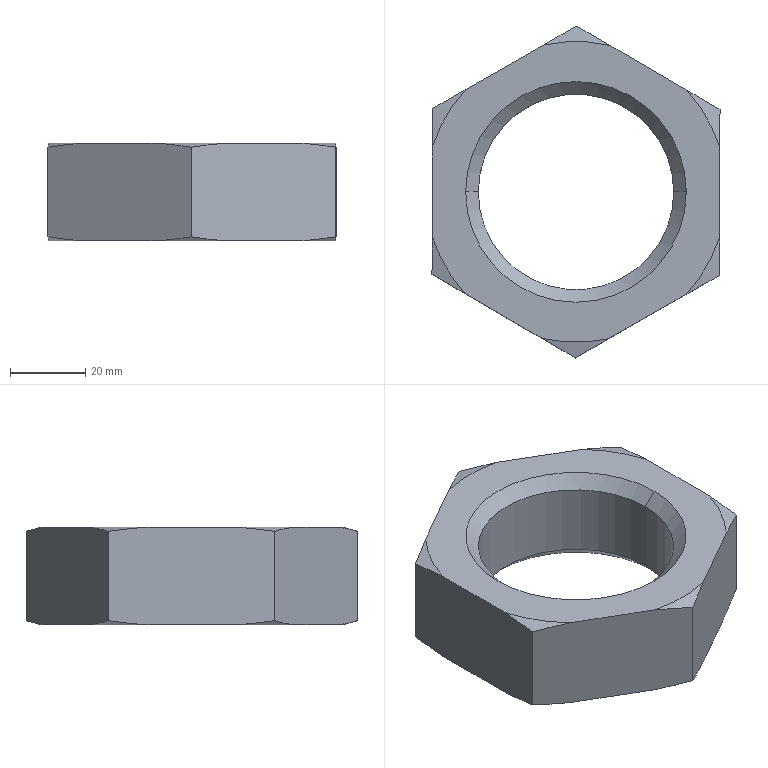Part | SolidWorks | features Cut 2, Chamfer 1, Extrusion 1 | 1 solid | 26 faces | box 76.6 x 88.249 x 26 mm | volume 74263 mm3 | cone 16 | plane 8 | cylinder 2 | commonest cylinder face diameters 52 x2
STEP:
#1=CARTESIAN_POINT('',(-26.,0.,22.662));
#2=VERTEX_POINT('',#1);
#3=CARTESIAN_POINT('',(26.,0.,22.662));
#4=VERTEX_POINT('',#3);
#5=CARTESIAN_POINT('',(0.,0.,22.662));
#6=DIRECTION('',(0.,0.,1.));
#7=DIRECTION('',(-1.,0.,0.));
#8=AXIS2_PLACEMENT_3D('',#5,#6,#7);
#9=CIRCLE('',#8,26.);
#10=EDGE_CURVE('',#2,#4,#9,.T.);
#11=ORIENTED_EDGE('',*,*,#10,.F.);
#12=CARTESIAN_POINT('',(-29.338,0.,26.));
#13=VERTEX_POINT('',#12);
#14=CARTESIAN_POINT('',(-26.,0.,22.662));
#15=DIRECTION('',(-0.7071,0.,0.7071));
#16=VECTOR('',#15,1000.);
#17=LINE('',#14,#16);
#18=EDGE_CURVE('',#2,#13,#17,.T.);
#19=ORIENTED_EDGE('',*,*,#18,.T.);
#20=CARTESIAN_POINT('',(29.338,0.,26.));
#21=VERTEX_POINT('',#20);
#22=CARTESIAN_POINT('',(0.,0.,26.));
#23=DIRECTION('',(0.,0.,-1.));
#24=DIRECTION('',(-1.,0.,0.));
#25=AXIS2_PLACEMENT_3D('',#22,#23,#24);
#26=CIRCLE('',#25,29.338);
#27=EDGE_CURVE('',#21,#13,#26,.T.);
#28=ORIENTED_EDGE('',*,*,#27,.F.);
#29=CARTESIAN_POINT('',(26.,0.,22.662));
#30=DIRECTION('',(0.7071,0.,0.7071));
#31=VECTOR('',#30,1000.);
#32=LINE('',#29,#31);
#33=EDGE_CURVE('',#4,#21,#32,.T.);
#34=ORIENTED_EDGE('',*,*,#33,.F.);
#35=EDGE_LOOP('',(#11,#19,#28,#34));
#36=FACE_OUTER_BOUND('',#35,.T.);
#37=CARTESIAN_POINT('',(0.,0.,22.662));
#38=DIRECTION('',(0.,0.,1.));
#39=DIRECTION('',(1.,0.,0.));
#40=AXIS2_PLACEMENT_3D('',#37,#38,#39);
#41=CONICAL_SURFACE('',#40,26.,0.7854);
#42=ADVANCED_FACE('',(#36),#41,.F.);
#43=CARTESIAN_POINT('',(26.,0.,3.338));
#44=VERTEX_POINT('',#43);
#45=CARTESIAN_POINT('',(-26.,0.,3.338));
#46=VERTEX_POINT('',#45);
#47=CARTESIAN_POINT('',(0.,0.,3.338));
#48=DIRECTION('',(0.,0.,-1.));
#49=DIRECTION('',(-1.,0.,0.));
#50=AXIS2_PLACEMENT_3D('',#47,#48,#49);
#51=CIRCLE('',#50,26.);
#52=EDGE_CURVE('',#44,#46,#51,.T.);
#53=ORIENTED_EDGE('',*,*,#52,.F.);
#54=CARTESIAN_POINT('',(29.338,0.,0.));
#55=VERTEX_POINT('',#54);
#56=CARTESIAN_POINT('',(29.338,0.,0.));
#57=DIRECTION('',(0.7071,0.,-0.7071));
#58=VECTOR('',#57,1000.);
#59=LINE('',#56,#58);
#60=EDGE_CURVE('',#44,#55,#59,.T.);
#61=ORIENTED_EDGE('',*,*,#60,.T.);
#62=CARTESIAN_POINT('',(-29.338,0.,0.));
#63=VERTEX_POINT('',#62);
#64=CARTESIAN_POINT('',(0.,0.,0.));
#65=DIRECTION('',(0.,0.,1.));
#66=DIRECTION('',(-1.,0.,0.));
#67=AXIS2_PLACEMENT_3D('',#64,#65,#66);
#68=CIRCLE('',#67,29.338);
#69=EDGE_CURVE('',#63,#55,#68,.T.);
#70=ORIENTED_EDGE('',*,*,#69,.F.);
#71=CARTESIAN_POINT('',(-29.338,0.,0.));
#72=DIRECTION('',(-0.7071,0.,-0.7071));
#73=VECTOR('',#72,1000.);
#74=LINE('',#71,#73);
#75=EDGE_CURVE('',#46,#63,#74,.T.);
#76=ORIENTED_EDGE('',*,*,#75,.F.);
#77=EDGE_LOOP('',(#53,#61,#70,#76));
#78=FACE_OUTER_BOUND('',#77,.T.);
#79=CARTESIAN_POINT('',(0.,0.,0.));
#80=DIRECTION('',(0.,0.,-1.));
#81=DIRECTION('',(-1.,0.,0.));
#82=AXIS2_PLACEMENT_3D('',#79,#80,#81);
#83=CONICAL_SURFACE('',#82,29.338,0.7854);
#84=ADVANCED_FACE('',(#78),#83,.F.);
#85=ORIENTED_EDGE('',*,*,#10,.T.);
#86=CARTESIAN_POINT('',(26.,0.,26.));
#87=DIRECTION('',(0.,0.,-1.));
#88=VECTOR('',#87,1000.);
#89=LINE('',#86,#88);
#90=EDGE_CURVE('',#4,#44,#89,.T.);
#91=ORIENTED_EDGE('',*,*,#90,.T.);
#92=ORIENTED_EDGE('',*,*,#52,.T.);
#93=CARTESIAN_POINT('',(-26.,0.,26.));
#94=DIRECTION('',(0.,0.,-1.));
#95=VECTOR('',#94,1000.);
#96=LINE('',#93,#95);
#97=EDGE_CURVE('',#2,#46,#96,.T.);
#98=ORIENTED_EDGE('',*,*,#97,.F.);
#99=EDGE_LOOP('',(#85,#91,#92,#98));
#100=FACE_OUTER_BOUND('',#99,.T.);
#101=CARTESIAN_POINT('',(0.,0.,26.));
#102=DIRECTION('',(0.,0.,-1.));
#103=DIRECTION('',(-1.,0.,0.));
#104=AXIS2_PLACEMENT_3D('',#101,#102,#103);
#105=CYLINDRICAL_SURFACE('',#104,26.);
#106=ADVANCED_FACE('',(#100),#105,.F.);
#107=CARTESIAN_POINT('',(38.3,21.912,24.895));
#108=VERTEX_POINT('',#107);
#109=CARTESIAN_POINT('',(29.451,27.068,26.));
#110=VERTEX_POINT('',#109);
#111=CARTESIAN_POINT('',(38.3,21.912,24.895));
#112=CARTESIAN_POINT('',(35.358,23.626,25.351));
#113=CARTESIAN_POINT('',(32.41,25.344,25.729));
#114=CARTESIAN_POINT('',(29.451,27.068,26.));
#115=B_SPLINE_CURVE_WITH_KNOTS('',3,(#111,#112,#113,#114),.UNSPECIFIED.,.F.,.F.,(4,4),(0.03608,0.04638),.UNSPECIFIED.);
#116=EDGE_CURVE('',#108,#110,#115,.T.);
#117=ORIENTED_EDGE('',*,*,#116,.F.);
#118=CARTESIAN_POINT('',(38.3,21.912,1.105));
#119=VERTEX_POINT('',#118);
#120=CARTESIAN_POINT('',(38.3,21.912,26.));
#121=DIRECTION('',(0.,0.,-1.));
#122=VECTOR('',#121,1000.);
#123=LINE('',#120,#122);
#124=EDGE_CURVE('',#108,#119,#123,.T.);
#125=ORIENTED_EDGE('',*,*,#124,.T.);
#126=CARTESIAN_POINT('',(29.451,27.068,0.));
#127=VERTEX_POINT('',#126);
#128=CARTESIAN_POINT('',(29.451,27.068,0.));
#129=CARTESIAN_POINT('',(30.931,26.205,0.1356));
#130=CARTESIAN_POINT('',(32.411,25.343,0.2982));
#131=CARTESIAN_POINT('',(35.36,23.625,0.6692));
#132=CARTESIAN_POINT('',(36.831,22.768,0.8776));
#133=CARTESIAN_POINT('',(38.3,21.912,1.105));
#134=B_SPLINE_CURVE_WITH_KNOTS('',3,(#128,#129,#130,#131,#132,#133),.UNSPECIFIED.,.F.,.F.,(4,2,4),(0.06989,0.07495,0.08001),.UNSPECIFIED.);
#135=EDGE_CURVE('',#127,#119,#134,.T.);
#136=ORIENTED_EDGE('',*,*,#135,.F.);
#137=CARTESIAN_POINT('',(9.023,38.969,0.));
#138=VERTEX_POINT('',#137);
#139=CARTESIAN_POINT('',(38.3,21.912,0.));
#140=DIRECTION('',(-0.8641,0.5034,0.));
#141=VECTOR('',#140,1000.);
#142=LINE('',#139,#141);
#143=EDGE_CURVE('',#127,#138,#142,.T.);
#144=ORIENTED_EDGE('',*,*,#143,.T.);
#145=CARTESIAN_POINT('',(0.1736,44.125,1.105));
#146=VERTEX_POINT('',#145);
#147=CARTESIAN_POINT('',(0.1736,44.125,1.105));
#148=CARTESIAN_POINT('',(3.115,42.411,0.6492));
#149=CARTESIAN_POINT('',(6.064,40.693,0.2712));
#150=CARTESIAN_POINT('',(9.023,38.969,0.));
#151=B_SPLINE_CURVE_WITH_KNOTS('',3,(#147,#148,#149,#150),.UNSPECIFIED.,.F.,.F.,(4,4),(0.03608,0.04638),.UNSPECIFIED.);
#152=EDGE_CURVE('',#146,#138,#151,.T.);
#153=ORIENTED_EDGE('',*,*,#152,.F.);
#154=CARTESIAN_POINT('',(0.1736,44.125,24.895));
#155=VERTEX_POINT('',#154);
#156=CARTESIAN_POINT('',(0.1736,44.125,26.));
#157=DIRECTION('',(0.,0.,-1.));
#158=VECTOR('',#157,1000.);
#159=LINE('',#156,#158);
#160=EDGE_CURVE('',#155,#146,#159,.T.);
#161=ORIENTED_EDGE('',*,*,#160,.F.);
#162=CARTESIAN_POINT('',(9.023,38.969,26.));
#163=VERTEX_POINT('',#162);
#164=CARTESIAN_POINT('',(9.023,38.969,26.));
#165=CARTESIAN_POINT('',(7.543,39.831,25.864));
#166=CARTESIAN_POINT('',(6.063,40.693,25.702));
#167=CARTESIAN_POINT('',(3.113,42.412,25.331));
#168=CARTESIAN_POINT('',(1.642,43.269,25.122));
#169=CARTESIAN_POINT('',(0.1736,44.125,24.895));
#170=B_SPLINE_CURVE_WITH_KNOTS('',3,(#164,#165,#166,#167,#168,#169),.UNSPECIFIED.,.F.,.F.,(4,2,4),(0.06989,0.07495,0.08001),.UNSPECIFIED.);
#171=EDGE_CURVE('',#163,#155,#170,.T.);
#172=ORIENTED_EDGE('',*,*,#171,.F.);
#173=CARTESIAN_POINT('',(38.3,21.912,26.));
#174=DIRECTION('',(-0.8641,0.5034,0.));
#175=VECTOR('',#174,1000.);
#176=LINE('',#173,#175);
#177=EDGE_CURVE('',#110,#163,#176,.T.);
#178=ORIENTED_EDGE('',*,*,#177,.F.);
#179=EDGE_LOOP('',(#117,#125,#136,#144,#153,#161,#172,#178));
#180=FACE_OUTER_BOUND('',#179,.T.);
#181=CARTESIAN_POINT('',(38.3,21.912,26.));
#182=DIRECTION('',(-0.5034,-0.8641,0.));
#183=DIRECTION('',(0.8641,-0.5034,0.));
#184=AXIS2_PLACEMENT_3D('',#181,#182,#183);
#185=PLANE('',#184);
#186=ADVANCED_FACE('',(#180),#185,.F.);
#187=CARTESIAN_POINT('',(-8.716,39.039,26.));
#188=VERTEX_POINT('',#187);
#189=CARTESIAN_POINT('',(0.1736,44.125,24.895));
#190=CARTESIAN_POINT('',(-2.781,42.434,25.351));
#191=CARTESIAN_POINT('',(-5.743,40.739,25.729));
#192=CARTESIAN_POINT('',(-8.716,39.039,26.));
#193=B_SPLINE_CURVE_WITH_KNOTS('',3,(#189,#190,#191,#192),.UNSPECIFIED.,.F.,.F.,(4,4),(0.03592,0.04622),.UNSPECIFIED.);
#194=EDGE_CURVE('',#155,#188,#193,.T.);
#195=ORIENTED_EDGE('',*,*,#194,.F.);
#196=ORIENTED_EDGE('',*,*,#160,.T.);
#197=CARTESIAN_POINT('',(-8.716,39.039,0.));
#198=VERTEX_POINT('',#197);
#199=CARTESIAN_POINT('',(-8.716,39.039,0.));
#200=CARTESIAN_POINT('',(-7.229,39.889,0.1356));
#201=CARTESIAN_POINT('',(-5.743,40.74,0.2982));
#202=CARTESIAN_POINT('',(-2.78,42.435,0.6692));
#203=CARTESIAN_POINT('',(-1.302,43.281,0.8776));
#204=CARTESIAN_POINT('',(0.1736,44.125,1.105));
#205=B_SPLINE_CURVE_WITH_KNOTS('',3,(#199,#200,#201,#202,#203,#204),.UNSPECIFIED.,.F.,.F.,(4,2,4),(0.06972,0.07478,0.07985),.UNSPECIFIED.);
#206=EDGE_CURVE('',#198,#146,#205,.T.);
#207=ORIENTED_EDGE('',*,*,#206,.F.);
#208=CARTESIAN_POINT('',(-29.237,27.298,0.));
#209=VERTEX_POINT('',#208);
#210=CARTESIAN_POINT('',(0.1736,44.125,0.));
#211=DIRECTION('',(-0.868,-0.4966,0.));
#212=VECTOR('',#211,1000.);
#213=LINE('',#210,#212);
#214=EDGE_CURVE('',#198,#209,#213,.T.);
#215=ORIENTED_EDGE('',*,*,#214,.T.);
#216=CARTESIAN_POINT('',(-38.126,22.213,1.105));
#217=VERTEX_POINT('',#216);
#218=CARTESIAN_POINT('',(-38.126,22.213,1.105));
#219=CARTESIAN_POINT('',(-35.171,23.903,0.6492));
#220=CARTESIAN_POINT('',(-32.209,25.598,0.2712));
#221=CARTESIAN_POINT('',(-29.237,27.298,0.));
#222=B_SPLINE_CURVE_WITH_KNOTS('',3,(#218,#219,#220,#221),.UNSPECIFIED.,.F.,.F.,(4,4),(0.03592,0.04622),.UNSPECIFIED.);
#223=EDGE_CURVE('',#217,#209,#222,.T.);
#224=ORIENTED_EDGE('',*,*,#223,.F.);
#225=CARTESIAN_POINT('',(-38.126,22.213,24.895));
#226=VERTEX_POINT('',#225);
#227=CARTESIAN_POINT('',(-38.126,22.213,26.));
#228=DIRECTION('',(0.,0.,-1.));
#229=VECTOR('',#228,1000.);
#230=LINE('',#227,#229);
#231=EDGE_CURVE('',#226,#217,#230,.T.);
#232=ORIENTED_EDGE('',*,*,#231,.F.);
#233=CARTESIAN_POINT('',(-29.237,27.298,26.));
#234=VERTEX_POINT('',#233);
#235=CARTESIAN_POINT('',(-29.237,27.298,26.));
#236=CARTESIAN_POINT('',(-30.723,26.448,25.864));
#237=CARTESIAN_POINT('',(-32.21,25.597,25.702));
#238=CARTESIAN_POINT('',(-35.173,23.902,25.331));
#239=CARTESIAN_POINT('',(-36.651,23.057,25.122));
#240=CARTESIAN_POINT('',(-38.126,22.213,24.895));
#241=B_SPLINE_CURVE_WITH_KNOTS('',3,(#235,#236,#237,#238,#239,#240),.UNSPECIFIED.,.F.,.F.,(4,2,4),(0.06972,0.07478,0.07985),.UNSPECIFIED.);
#242=EDGE_CURVE('',#234,#226,#241,.T.);
#243=ORIENTED_EDGE('',*,*,#242,.F.);
#244=CARTESIAN_POINT('',(0.1736,44.125,26.));
#245=DIRECTION('',(-0.868,-0.4966,0.));
#246=VECTOR('',#245,1000.);
#247=LINE('',#244,#246);
#248=EDGE_CURVE('',#188,#234,#247,.T.);
#249=ORIENTED_EDGE('',*,*,#248,.F.);
#250=EDGE_LOOP('',(#195,#196,#207,#215,#224,#232,#243,#249));
#251=FACE_OUTER_BOUND('',#250,.T.);
#252=CARTESIAN_POINT('',(0.1736,44.125,26.));
#253=DIRECTION('',(0.4966,-0.868,0.));
#254=DIRECTION('',(0.868,0.4966,0.));
#255=AXIS2_PLACEMENT_3D('',#252,#253,#254);
#256=PLANE('',#255);
#257=ADVANCED_FACE('',(#251),#256,.F.);
#258=CARTESIAN_POINT('',(-38.167,11.971,26.));
#259=VERTEX_POINT('',#258);
#260=CARTESIAN_POINT('',(-38.126,22.213,24.895));
#261=CARTESIAN_POINT('',(-38.14,18.808,25.351));
#262=CARTESIAN_POINT('',(-38.153,15.395,25.729));
#263=CARTESIAN_POINT('',(-38.167,11.971,26.));
#264=B_SPLINE_CURVE_WITH_KNOTS('',3,(#260,#261,#262,#263),.UNSPECIFIED.,.F.,.F.,(4,4),(0.03114,0.04144),.UNSPECIFIED.);
#265=EDGE_CURVE('',#226,#259,#264,.T.);
#266=ORIENTED_EDGE('',*,*,#265,.F.);
#267=ORIENTED_EDGE('',*,*,#231,.T.);
#268=CARTESIAN_POINT('',(-38.167,11.971,0.));
#269=VERTEX_POINT('',#268);
#270=CARTESIAN_POINT('',(-38.167,11.971,0.));
#271=CARTESIAN_POINT('',(-38.16,13.682,0.1355));
#272=CARTESIAN_POINT('',(-38.153,15.395,0.2981));
#273=CARTESIAN_POINT('',(-38.14,18.809,0.6691));
#274=CARTESIAN_POINT('',(-38.133,20.513,0.8775));
#275=CARTESIAN_POINT('',(-38.126,22.213,1.105));
#276=B_SPLINE_CURVE_WITH_KNOTS('',3,(#270,#271,#272,#273,#274,#275),.UNSPECIFIED.,.F.,.F.,(4,2,4),(0.06496,0.07003,0.0751),.UNSPECIFIED.);
#277=EDGE_CURVE('',#269,#217,#276,.T.);
#278=ORIENTED_EDGE('',*,*,#277,.F.);
#279=CARTESIAN_POINT('',(-38.26,-11.671,0.));
#280=VERTEX_POINT('',#279);
#281=CARTESIAN_POINT('',(-38.126,22.213,0.));
#282=DIRECTION('',(-0.003934,-1.,0.));
#283=VECTOR('',#282,1000.);
#284=LINE('',#281,#283);
#285=EDGE_CURVE('',#269,#280,#284,.T.);
#286=ORIENTED_EDGE('',*,*,#285,.T.);
#287=CARTESIAN_POINT('',(-38.3,-21.912,1.105));
#288=VERTEX_POINT('',#287);
#289=CARTESIAN_POINT('',(-38.3,-21.912,1.105));
#290=CARTESIAN_POINT('',(-38.286,-18.507,0.6491));
#291=CARTESIAN_POINT('',(-38.273,-15.094,0.2711));
#292=CARTESIAN_POINT('',(-38.26,-11.671,0.));
#293=B_SPLINE_CURVE_WITH_KNOTS('',3,(#289,#290,#291,#292),.UNSPECIFIED.,.F.,.F.,(4,4),(0.03114,0.04144),.UNSPECIFIED.);
#294=EDGE_CURVE('',#288,#280,#293,.T.);
#295=ORIENTED_EDGE('',*,*,#294,.F.);
#296=CARTESIAN_POINT('',(-38.3,-21.912,24.895));
#297=VERTEX_POINT('',#296);
#298=CARTESIAN_POINT('',(-38.3,-21.912,26.));
#299=DIRECTION('',(0.,0.,-1.));
#300=VECTOR('',#299,1000.);
#301=LINE('',#298,#300);
#302=EDGE_CURVE('',#297,#288,#301,.T.);
#303=ORIENTED_EDGE('',*,*,#302,.F.);
#304=CARTESIAN_POINT('',(-38.26,-11.671,26.));
#305=VERTEX_POINT('',#304);
#306=CARTESIAN_POINT('',(-38.26,-11.671,26.));
#307=CARTESIAN_POINT('',(-38.266,-13.381,25.865));
#308=CARTESIAN_POINT('',(-38.273,-15.095,25.702));
#309=CARTESIAN_POINT('',(-38.286,-18.509,25.331));
#310=CARTESIAN_POINT('',(-38.293,-20.212,25.122));
#311=CARTESIAN_POINT('',(-38.3,-21.912,24.895));
#312=B_SPLINE_CURVE_WITH_KNOTS('',3,(#306,#307,#308,#309,#310,#311),.UNSPECIFIED.,.F.,.F.,(4,2,4),(0.06496,0.07003,0.0751),.UNSPECIFIED.);
#313=EDGE_CURVE('',#305,#297,#312,.T.);
#314=ORIENTED_EDGE('',*,*,#313,.F.);
#315=CARTESIAN_POINT('',(-38.126,22.213,26.));
#316=DIRECTION('',(-0.003934,-1.,0.));
#317=VECTOR('',#316,1000.);
#318=LINE('',#315,#317);
#319=EDGE_CURVE('',#259,#305,#318,.T.);
#320=ORIENTED_EDGE('',*,*,#319,.F.);
#321=EDGE_LOOP('',(#266,#267,#278,#286,#295,#303,#314,#320));
#322=FACE_OUTER_BOUND('',#321,.T.);
#323=CARTESIAN_POINT('',(-38.126,22.213,26.));
#324=DIRECTION('',(1.,-0.003934,0.));
#325=DIRECTION('',(0.003934,1.,0.));
#326=AXIS2_PLACEMENT_3D('',#323,#324,#325);
#327=PLANE('',#326);
#328=ADVANCED_FACE('',(#322),#327,.F.);
#329=CARTESIAN_POINT('',(-29.451,-27.068,26.));
#330=VERTEX_POINT('',#329);
#331=CARTESIAN_POINT('',(-38.3,-21.912,24.895));
#332=CARTESIAN_POINT('',(-35.358,-23.626,25.351));
#333=CARTESIAN_POINT('',(-32.41,-25.344,25.729));
#334=CARTESIAN_POINT('',(-29.451,-27.068,26.));
#335=B_SPLINE_CURVE_WITH_KNOTS('',3,(#331,#332,#333,#334),.UNSPECIFIED.,.F.,.F.,(4,4),(0.03608,0.04638),.UNSPECIFIED.);
#336=EDGE_CURVE('',#297,#330,#335,.T.);
#337=ORIENTED_EDGE('',*,*,#336,.F.);
#338=ORIENTED_EDGE('',*,*,#302,.T.);
#339=CARTESIAN_POINT('',(-29.451,-27.068,0.));
#340=VERTEX_POINT('',#339);
#341=CARTESIAN_POINT('',(-29.451,-27.068,0.));
#342=CARTESIAN_POINT('',(-30.931,-26.205,0.1356));
#343=CARTESIAN_POINT('',(-32.411,-25.343,0.2982));
#344=CARTESIAN_POINT('',(-35.36,-23.625,0.6692));
#345=CARTESIAN_POINT('',(-36.831,-22.768,0.8776));
#346=CARTESIAN_POINT('',(-38.3,-21.912,1.105));
#347=B_SPLINE_CURVE_WITH_KNOTS('',3,(#341,#342,#343,#344,#345,#346),.UNSPECIFIED.,.F.,.F.,(4,2,4),(0.06989,0.07495,0.08001),.UNSPECIFIED.);
#348=EDGE_CURVE('',#340,#288,#347,.T.);
#349=ORIENTED_EDGE('',*,*,#348,.F.);
#350=CARTESIAN_POINT('',(-9.023,-38.969,0.));
#351=VERTEX_POINT('',#350);
#352=CARTESIAN_POINT('',(-38.3,-21.912,0.));
#353=DIRECTION('',(0.8641,-0.5034,0.));
#354=VECTOR('',#353,1000.);
#355=LINE('',#352,#354);
#356=EDGE_CURVE('',#340,#351,#355,.T.);
#357=ORIENTED_EDGE('',*,*,#356,.T.);
#358=CARTESIAN_POINT('',(-0.1736,-44.125,1.105));
#359=VERTEX_POINT('',#358);
#360=CARTESIAN_POINT('',(-0.1736,-44.125,1.105));
#361=CARTESIAN_POINT('',(-3.115,-42.411,0.6492));
#362=CARTESIAN_POINT('',(-6.064,-40.693,0.2712));
#363=CARTESIAN_POINT('',(-9.023,-38.969,0.));
#364=B_SPLINE_CURVE_WITH_KNOTS('',3,(#360,#361,#362,#363),.UNSPECIFIED.,.F.,.F.,(4,4),(0.03608,0.04638),.UNSPECIFIED.);
#365=EDGE_CURVE('',#359,#351,#364,.T.);
#366=ORIENTED_EDGE('',*,*,#365,.F.);
#367=CARTESIAN_POINT('',(-0.1736,-44.125,24.895));
#368=VERTEX_POINT('',#367);
#369=CARTESIAN_POINT('',(-0.1736,-44.125,26.));
#370=DIRECTION('',(0.,0.,-1.));
#371=VECTOR('',#370,1000.);
#372=LINE('',#369,#371);
#373=EDGE_CURVE('',#368,#359,#372,.T.);
#374=ORIENTED_EDGE('',*,*,#373,.F.);
#375=CARTESIAN_POINT('',(-9.023,-38.969,26.));
#376=VERTEX_POINT('',#375);
#377=CARTESIAN_POINT('',(-9.023,-38.969,26.));
#378=CARTESIAN_POINT('',(-7.543,-39.831,25.864));
#379=CARTESIAN_POINT('',(-6.063,-40.693,25.702));
#380=CARTESIAN_POINT('',(-3.113,-42.412,25.331));
#381=CARTESIAN_POINT('',(-1.642,-43.269,25.122));
#382=CARTESIAN_POINT('',(-0.1736,-44.125,24.895));
#383=B_SPLINE_CURVE_WITH_KNOTS('',3,(#377,#378,#379,#380,#381,#382),.UNSPECIFIED.,.F.,.F.,(4,2,4),(0.06989,0.07495,0.08001),.UNSPECIFIED.);
#384=EDGE_CURVE('',#376,#368,#383,.T.);
#385=ORIENTED_EDGE('',*,*,#384,.F.);
#386=CARTESIAN_POINT('',(-38.3,-21.912,26.));
#387=DIRECTION('',(0.8641,-0.5034,0.));
#388=VECTOR('',#387,1000.);
#389=LINE('',#386,#388);
#390=EDGE_CURVE('',#330,#376,#389,.T.);
#391=ORIENTED_EDGE('',*,*,#390,.F.);
#392=EDGE_LOOP('',(#337,#338,#349,#357,#366,#374,#385,#391));
#393=FACE_OUTER_BOUND('',#392,.T.);
#394=CARTESIAN_POINT('',(-38.3,-21.912,26.));
#395=DIRECTION('',(0.5034,0.8641,0.));
#396=DIRECTION('',(-0.8641,0.5034,0.));
#397=AXIS2_PLACEMENT_3D('',#394,#395,#396);
#398=PLANE('',#397);
#399=ADVANCED_FACE('',(#393),#398,.F.);
#400=CARTESIAN_POINT('',(8.716,-39.039,26.));
#401=VERTEX_POINT('',#400);
#402=CARTESIAN_POINT('',(-0.1736,-44.125,24.895));
#403=CARTESIAN_POINT('',(2.781,-42.434,25.351));
#404=CARTESIAN_POINT('',(5.743,-40.739,25.729));
#405=CARTESIAN_POINT('',(8.716,-39.039,26.));
#406=B_SPLINE_CURVE_WITH_KNOTS('',3,(#402,#403,#404,#405),.UNSPECIFIED.,.F.,.F.,(4,4),(0.03592,0.04622),.UNSPECIFIED.);
#407=EDGE_CURVE('',#368,#401,#406,.T.);
#408=ORIENTED_EDGE('',*,*,#407,.F.);
#409=ORIENTED_EDGE('',*,*,#373,.T.);
#410=CARTESIAN_POINT('',(8.716,-39.039,0.));
#411=VERTEX_POINT('',#410);
#412=CARTESIAN_POINT('',(8.716,-39.039,0.));
#413=CARTESIAN_POINT('',(7.229,-39.889,0.1356));
#414=CARTESIAN_POINT('',(5.743,-40.74,0.2982));
#415=CARTESIAN_POINT('',(2.78,-42.435,0.6692));
#416=CARTESIAN_POINT('',(1.302,-43.281,0.8776));
#417=CARTESIAN_POINT('',(-0.1736,-44.125,1.105));
#418=B_SPLINE_CURVE_WITH_KNOTS('',3,(#412,#413,#414,#415,#416,#417),.UNSPECIFIED.,.F.,.F.,(4,2,4),(0.06972,0.07478,0.07985),.UNSPECIFIED.);
#419=EDGE_CURVE('',#411,#359,#418,.T.);
#420=ORIENTED_EDGE('',*,*,#419,.F.);
#421=CARTESIAN_POINT('',(29.237,-27.298,0.));
#422=VERTEX_POINT('',#421);
#423=CARTESIAN_POINT('',(-0.1736,-44.125,0.));
#424=DIRECTION('',(0.868,0.4966,0.));
#425=VECTOR('',#424,1000.);
#426=LINE('',#423,#425);
#427=EDGE_CURVE('',#411,#422,#426,.T.);
#428=ORIENTED_EDGE('',*,*,#427,.T.);
#429=CARTESIAN_POINT('',(38.126,-22.213,1.105));
#430=VERTEX_POINT('',#429);
#431=CARTESIAN_POINT('',(38.126,-22.213,1.105));
#432=CARTESIAN_POINT('',(35.171,-23.903,0.6492));
#433=CARTESIAN_POINT('',(32.209,-25.598,0.2712));
#434=CARTESIAN_POINT('',(29.237,-27.298,0.));
#435=B_SPLINE_CURVE_WITH_KNOTS('',3,(#431,#432,#433,#434),.UNSPECIFIED.,.F.,.F.,(4,4),(0.03592,0.04622),.UNSPECIFIED.);
#436=EDGE_CURVE('',#430,#422,#435,.T.);
#437=ORIENTED_EDGE('',*,*,#436,.F.);
#438=CARTESIAN_POINT('',(38.126,-22.213,24.895));
#439=VERTEX_POINT('',#438);
#440=CARTESIAN_POINT('',(38.126,-22.213,26.));
#441=DIRECTION('',(0.,0.,-1.));
#442=VECTOR('',#441,1000.);
#443=LINE('',#440,#442);
#444=EDGE_CURVE('',#439,#430,#443,.T.);
#445=ORIENTED_EDGE('',*,*,#444,.F.);
#446=CARTESIAN_POINT('',(29.237,-27.298,26.));
#447=VERTEX_POINT('',#446);
#448=CARTESIAN_POINT('',(29.237,-27.298,26.));
#449=CARTESIAN_POINT('',(30.723,-26.448,25.864));
#450=CARTESIAN_POINT('',(32.21,-25.597,25.702));
#451=CARTESIAN_POINT('',(35.173,-23.902,25.331));
#452=CARTESIAN_POINT('',(36.651,-23.057,25.122));
#453=CARTESIAN_POINT('',(38.126,-22.213,24.895));
#454=B_SPLINE_CURVE_WITH_KNOTS('',3,(#448,#449,#450,#451,#452,#453),.UNSPECIFIED.,.F.,.F.,(4,2,4),(0.06972,0.07478,0.07985),.UNSPECIFIED.);
#455=EDGE_CURVE('',#447,#439,#454,.T.);
#456=ORIENTED_EDGE('',*,*,#455,.F.);
#457=CARTESIAN_POINT('',(-0.1736,-44.125,26.));
#458=DIRECTION('',(0.868,0.4966,0.));
#459=VECTOR('',#458,1000.);
#460=LINE('',#457,#459);
#461=EDGE_CURVE('',#401,#447,#460,.T.);
#462=ORIENTED_EDGE('',*,*,#461,.F.);
#463=EDGE_LOOP('',(#408,#409,#420,#428,#437,#445,#456,#462));
#464=FACE_OUTER_BOUND('',#463,.T.);
#465=CARTESIAN_POINT('',(-0.1736,-44.125,26.));
#466=DIRECTION('',(-0.4966,0.868,0.));
#467=DIRECTION('',(-0.868,-0.4966,0.));
#468=AXIS2_PLACEMENT_3D('',#465,#466,#467);
#469=PLANE('',#468);
#470=ADVANCED_FACE('',(#464),#469,.F.);
#471=CARTESIAN_POINT('',(38.167,-11.971,26.));
#472=VERTEX_POINT('',#471);
#473=CARTESIAN_POINT('',(38.126,-22.213,24.895));
#474=CARTESIAN_POINT('',(38.14,-18.808,25.351));
#475=CARTESIAN_POINT('',(38.153,-15.395,25.729));
#476=CARTESIAN_POINT('',(38.167,-11.971,26.));
#477=B_SPLINE_CURVE_WITH_KNOTS('',3,(#473,#474,#475,#476),.UNSPECIFIED.,.F.,.F.,(4,4),(0.03114,0.04144),.UNSPECIFIED.);
#478=EDGE_CURVE('',#439,#472,#477,.T.);
#479=ORIENTED_EDGE('',*,*,#478,.F.);
#480=ORIENTED_EDGE('',*,*,#444,.T.);
#481=CARTESIAN_POINT('',(38.167,-11.971,0.));
#482=VERTEX_POINT('',#481);
#483=CARTESIAN_POINT('',(38.167,-11.971,0.));
#484=CARTESIAN_POINT('',(38.16,-13.682,0.1355));
#485=CARTESIAN_POINT('',(38.153,-15.395,0.2981));
#486=CARTESIAN_POINT('',(38.14,-18.809,0.6691));
#487=CARTESIAN_POINT('',(38.133,-20.513,0.8775));
#488=CARTESIAN_POINT('',(38.126,-22.213,1.105));
#489=B_SPLINE_CURVE_WITH_KNOTS('',3,(#483,#484,#485,#486,#487,#488),.UNSPECIFIED.,.F.,.F.,(4,2,4),(0.06496,0.07003,0.0751),.UNSPECIFIED.);
#490=EDGE_CURVE('',#482,#430,#489,.T.);
#491=ORIENTED_EDGE('',*,*,#490,.F.);
#492=CARTESIAN_POINT('',(38.26,11.671,0.));
#493=VERTEX_POINT('',#492);
#494=CARTESIAN_POINT('',(38.126,-22.213,0.));
#495=DIRECTION('',(0.003934,1.,0.));
#496=VECTOR('',#495,1000.);
#497=LINE('',#494,#496);
#498=EDGE_CURVE('',#482,#493,#497,.T.);
#499=ORIENTED_EDGE('',*,*,#498,.T.);
#500=CARTESIAN_POINT('',(38.3,21.912,1.105));
#501=CARTESIAN_POINT('',(38.286,18.507,0.6491));
#502=CARTESIAN_POINT('',(38.273,15.094,0.2711));
#503=CARTESIAN_POINT('',(38.26,11.671,0.));
#504=B_SPLINE_CURVE_WITH_KNOTS('',3,(#500,#501,#502,#503),.UNSPECIFIED.,.F.,.F.,(4,4),(0.03114,0.04144),.UNSPECIFIED.);
#505=EDGE_CURVE('',#119,#493,#504,.T.);
#506=ORIENTED_EDGE('',*,*,#505,.F.);
#507=ORIENTED_EDGE('',*,*,#124,.F.);
#508=CARTESIAN_POINT('',(38.26,11.671,26.));
#509=VERTEX_POINT('',#508);
#510=CARTESIAN_POINT('',(38.26,11.671,26.));
#511=CARTESIAN_POINT('',(38.266,13.381,25.865));
#512=CARTESIAN_POINT('',(38.273,15.095,25.702));
#513=CARTESIAN_POINT('',(38.286,18.509,25.331));
#514=CARTESIAN_POINT('',(38.293,20.212,25.122));
#515=CARTESIAN_POINT('',(38.3,21.912,24.895));
#516=B_SPLINE_CURVE_WITH_KNOTS('',3,(#510,#511,#512,#513,#514,#515),.UNSPECIFIED.,.F.,.F.,(4,2,4),(0.06496,0.07003,0.0751),.UNSPECIFIED.);
#517=EDGE_CURVE('',#509,#108,#516,.T.);
#518=ORIENTED_EDGE('',*,*,#517,.F.);
#519=CARTESIAN_POINT('',(38.126,-22.213,26.));
#520=DIRECTION('',(0.003934,1.,0.));
#521=VECTOR('',#520,1000.);
#522=LINE('',#519,#521);
#523=EDGE_CURVE('',#472,#509,#522,.T.);
#524=ORIENTED_EDGE('',*,*,#523,.F.);
#525=EDGE_LOOP('',(#479,#480,#491,#499,#506,#507,#518,#524));
#526=FACE_OUTER_BOUND('',#525,.T.);
#527=CARTESIAN_POINT('',(38.126,-22.213,26.));
#528=DIRECTION('',(-1.,0.003934,0.));
#529=DIRECTION('',(-0.003934,-1.,0.));
#530=AXIS2_PLACEMENT_3D('',#527,#528,#529);
#531=PLANE('',#530);
#532=ADVANCED_FACE('',(#526),#531,.F.);
#533=ORIENTED_EDGE('',*,*,#27,.T.);
#534=CARTESIAN_POINT('',(0.,0.,26.));
#535=DIRECTION('',(0.,0.,-1.));
#536=DIRECTION('',(-1.,0.,0.));
#537=AXIS2_PLACEMENT_3D('',#534,#535,#536);
#538=CIRCLE('',#537,29.338);
#539=EDGE_CURVE('',#13,#21,#538,.T.);
#540=ORIENTED_EDGE('',*,*,#539,.T.);
#541=EDGE_LOOP('',(#533,#540));
#542=FACE_BOUND('',#541,.T.);
#543=CARTESIAN_POINT('',(0.,0.,26.));
#544=DIRECTION('',(0.,0.,-1.));
#545=DIRECTION('',(-1.,0.,0.));
#546=AXIS2_PLACEMENT_3D('',#543,#544,#545);
#547=CIRCLE('',#546,40.);
#548=EDGE_CURVE('',#259,#234,#547,.T.);
#549=ORIENTED_EDGE('',*,*,#548,.F.);
#550=ORIENTED_EDGE('',*,*,#319,.T.);
#551=CARTESIAN_POINT('',(0.,0.,26.));
#552=DIRECTION('',(0.,0.,-1.));
#553=DIRECTION('',(-1.,0.,0.));
#554=AXIS2_PLACEMENT_3D('',#551,#552,#553);
#555=CIRCLE('',#554,40.);
#556=EDGE_CURVE('',#330,#305,#555,.T.);
#557=ORIENTED_EDGE('',*,*,#556,.F.);
#558=ORIENTED_EDGE('',*,*,#390,.T.);
#559=CARTESIAN_POINT('',(0.,0.,26.));
#560=DIRECTION('',(0.,0.,-1.));
#561=DIRECTION('',(-1.,0.,0.));
#562=AXIS2_PLACEMENT_3D('',#559,#560,#561);
#563=CIRCLE('',#562,40.);
#564=EDGE_CURVE('',#401,#376,#563,.T.);
#565=ORIENTED_EDGE('',*,*,#564,.F.);
#566=ORIENTED_EDGE('',*,*,#461,.T.);
#567=CARTESIAN_POINT('',(0.,0.,26.));
#568=DIRECTION('',(0.,0.,-1.));
#569=DIRECTION('',(-1.,0.,0.));
#570=AXIS2_PLACEMENT_3D('',#567,#568,#569);
#571=CIRCLE('',#570,40.);
#572=EDGE_CURVE('',#472,#447,#571,.T.);
#573=ORIENTED_EDGE('',*,*,#572,.F.);
#574=ORIENTED_EDGE('',*,*,#523,.T.);
#575=CARTESIAN_POINT('',(0.,0.,26.));
#576=DIRECTION('',(0.,0.,1.));
#577=DIRECTION('',(1.,0.,0.));
#578=AXIS2_PLACEMENT_3D('',#575,#576,#577);
#579=CIRCLE('',#578,40.);
#580=EDGE_CURVE('',#509,#110,#579,.T.);
#581=ORIENTED_EDGE('',*,*,#580,.T.);
#582=ORIENTED_EDGE('',*,*,#177,.T.);
#583=CARTESIAN_POINT('',(0.,0.,26.));
#584=DIRECTION('',(0.,0.,-1.));
#585=DIRECTION('',(-1.,0.,0.));
#586=AXIS2_PLACEMENT_3D('',#583,#584,#585);
#587=CIRCLE('',#586,40.);
#588=EDGE_CURVE('',#188,#163,#587,.T.);
#589=ORIENTED_EDGE('',*,*,#588,.F.);
#590=ORIENTED_EDGE('',*,*,#248,.T.);
#591=EDGE_LOOP('',(#549,#550,#557,#558,#565,#566,#573,#574,#581,#582,#589,#590));
#592=FACE_OUTER_BOUND('',#591,.T.);
#593=CARTESIAN_POINT('',(76.426,-0.3006,26.));
#594=DIRECTION('',(0.,0.,-1.));
#595=DIRECTION('',(-1.,0.,0.));
#596=AXIS2_PLACEMENT_3D('',#593,#594,#595);
#597=PLANE('',#596);
#598=ADVANCED_FACE('',(#542,#592),#597,.F.);
#599=ORIENTED_EDGE('',*,*,#69,.T.);
#600=CARTESIAN_POINT('',(0.,0.,0.));
#601=DIRECTION('',(0.,0.,1.));
#602=DIRECTION('',(-1.,0.,0.));
#603=AXIS2_PLACEMENT_3D('',#600,#601,#602);
#604=CIRCLE('',#603,29.338);
#605=EDGE_CURVE('',#55,#63,#604,.T.);
#606=ORIENTED_EDGE('',*,*,#605,.T.);
#607=EDGE_LOOP('',(#599,#606));
#608=FACE_BOUND('',#607,.T.);
#609=ORIENTED_EDGE('',*,*,#285,.F.);
#610=CARTESIAN_POINT('',(0.,0.,0.));
#611=DIRECTION('',(0.,0.,-1.));
#612=DIRECTION('',(-1.,0.,0.));
#613=AXIS2_PLACEMENT_3D('',#610,#611,#612);
#614=CIRCLE('',#613,40.);
#615=EDGE_CURVE('',#269,#209,#614,.T.);
#616=ORIENTED_EDGE('',*,*,#615,.T.);
#617=ORIENTED_EDGE('',*,*,#214,.F.);
#618=CARTESIAN_POINT('',(0.,0.,0.));
#619=DIRECTION('',(0.,0.,-1.));
#620=DIRECTION('',(-1.,0.,0.));
#621=AXIS2_PLACEMENT_3D('',#618,#619,#620);
#622=CIRCLE('',#621,40.);
#623=EDGE_CURVE('',#198,#138,#622,.T.);
#624=ORIENTED_EDGE('',*,*,#623,.T.);
#625=ORIENTED_EDGE('',*,*,#143,.F.);
#626=CARTESIAN_POINT('',(0.,0.,0.));
#627=DIRECTION('',(0.,0.,-1.));
#628=DIRECTION('',(-1.,0.,0.));
#629=AXIS2_PLACEMENT_3D('',#626,#627,#628);
#630=CIRCLE('',#629,40.);
#631=EDGE_CURVE('',#127,#493,#630,.T.);
#632=ORIENTED_EDGE('',*,*,#631,.T.);
#633=ORIENTED_EDGE('',*,*,#498,.F.);
#634=CARTESIAN_POINT('',(0.,0.,0.));
#635=DIRECTION('',(0.,0.,-1.));
#636=DIRECTION('',(-1.,0.,0.));
#637=AXIS2_PLACEMENT_3D('',#634,#635,#636);
#638=CIRCLE('',#637,40.);
#639=EDGE_CURVE('',#482,#422,#638,.T.);
#640=ORIENTED_EDGE('',*,*,#639,.T.);
#641=ORIENTED_EDGE('',*,*,#427,.F.);
#642=CARTESIAN_POINT('',(0.,0.,0.));
#643=DIRECTION('',(0.,0.,-1.));
#644=DIRECTION('',(-1.,0.,0.));
#645=AXIS2_PLACEMENT_3D('',#642,#643,#644);
#646=CIRCLE('',#645,40.);
#647=EDGE_CURVE('',#411,#351,#646,.T.);
#648=ORIENTED_EDGE('',*,*,#647,.T.);
#649=ORIENTED_EDGE('',*,*,#356,.F.);
#650=CARTESIAN_POINT('',(0.,0.,0.));
#651=DIRECTION('',(0.,0.,-1.));
#652=DIRECTION('',(-1.,0.,0.));
#653=AXIS2_PLACEMENT_3D('',#650,#651,#652);
#654=CIRCLE('',#653,40.);
#655=EDGE_CURVE('',#340,#280,#654,.T.);
#656=ORIENTED_EDGE('',*,*,#655,.T.);
#657=EDGE_LOOP('',(#609,#616,#617,#624,#625,#632,#633,#640,#641,#648,#649,#656));
#658=FACE_OUTER_BOUND('',#657,.T.);
#659=CARTESIAN_POINT('',(76.426,-0.3006,0.));
#660=DIRECTION('',(0.,0.,-1.));
#661=DIRECTION('',(-1.,0.,0.));
#662=AXIS2_PLACEMENT_3D('',#659,#660,#661);
#663=PLANE('',#662);
#664=ADVANCED_FACE('',(#608,#658),#663,.T.);
#665=ORIENTED_EDGE('',*,*,#90,.F.);
#666=CARTESIAN_POINT('',(0.,0.,22.662));
#667=DIRECTION('',(0.,0.,1.));
#668=DIRECTION('',(-1.,0.,0.));
#669=AXIS2_PLACEMENT_3D('',#666,#667,#668);
#670=CIRCLE('',#669,26.);
#671=EDGE_CURVE('',#4,#2,#670,.T.);
#672=ORIENTED_EDGE('',*,*,#671,.T.);
#673=ORIENTED_EDGE('',*,*,#97,.T.);
#674=CARTESIAN_POINT('',(0.,0.,3.338));
#675=DIRECTION('',(0.,0.,-1.));
#676=DIRECTION('',(-1.,0.,0.));
#677=AXIS2_PLACEMENT_3D('',#674,#675,#676);
#678=CIRCLE('',#677,26.);
#679=EDGE_CURVE('',#46,#44,#678,.T.);
#680=ORIENTED_EDGE('',*,*,#679,.T.);
#681=EDGE_LOOP('',(#665,#672,#673,#680));
#682=FACE_OUTER_BOUND('',#681,.T.);
#683=CARTESIAN_POINT('',(0.,0.,26.));
#684=DIRECTION('',(0.,0.,-1.));
#685=DIRECTION('',(-1.,0.,0.));
#686=AXIS2_PLACEMENT_3D('',#683,#684,#685);
#687=CYLINDRICAL_SURFACE('',#686,26.);
#688=ADVANCED_FACE('',(#682),#687,.F.);
#689=ORIENTED_EDGE('',*,*,#436,.T.);
#690=ORIENTED_EDGE('',*,*,#639,.F.);
#691=ORIENTED_EDGE('',*,*,#490,.T.);
#692=EDGE_LOOP('',(#689,#690,#691));
#693=FACE_OUTER_BOUND('',#692,.T.);
#694=CARTESIAN_POINT('',(0.,0.,0.));
#695=DIRECTION('',(0.,0.,1.));
#696=DIRECTION('',(-1.,0.,0.));
#697=AXIS2_PLACEMENT_3D('',#694,#695,#696);
#698=CONICAL_SURFACE('',#697,40.,1.309);
#699=ADVANCED_FACE('',(#693),#698,.T.);
#700=ORIENTED_EDGE('',*,*,#135,.T.);
#701=ORIENTED_EDGE('',*,*,#505,.T.);
#702=ORIENTED_EDGE('',*,*,#631,.F.);
#703=EDGE_LOOP('',(#700,#701,#702));
#704=FACE_OUTER_BOUND('',#703,.T.);
#705=CARTESIAN_POINT('',(0.,0.,0.));
#706=DIRECTION('',(0.,0.,1.));
#707=DIRECTION('',(-1.,0.,0.));
#708=AXIS2_PLACEMENT_3D('',#705,#706,#707);
#709=CONICAL_SURFACE('',#708,40.,1.309);
#710=ADVANCED_FACE('',(#704),#709,.T.);
#711=ORIENTED_EDGE('',*,*,#365,.T.);
#712=ORIENTED_EDGE('',*,*,#647,.F.);
#713=ORIENTED_EDGE('',*,*,#419,.T.);
#714=EDGE_LOOP('',(#711,#712,#713));
#715=FACE_OUTER_BOUND('',#714,.T.);
#716=CARTESIAN_POINT('',(0.,0.,0.));
#717=DIRECTION('',(0.,0.,1.));
#718=DIRECTION('',(-1.,0.,0.));
#719=AXIS2_PLACEMENT_3D('',#716,#717,#718);
#720=CONICAL_SURFACE('',#719,40.,1.309);
#721=ADVANCED_FACE('',(#715),#720,.T.);
#722=ORIENTED_EDGE('',*,*,#294,.T.);
#723=ORIENTED_EDGE('',*,*,#655,.F.);
#724=ORIENTED_EDGE('',*,*,#348,.T.);
#725=EDGE_LOOP('',(#722,#723,#724));
#726=FACE_OUTER_BOUND('',#725,.T.);
#727=CARTESIAN_POINT('',(0.,0.,0.));
#728=DIRECTION('',(0.,0.,1.));
#729=DIRECTION('',(-1.,0.,0.));
#730=AXIS2_PLACEMENT_3D('',#727,#728,#729);
#731=CONICAL_SURFACE('',#730,40.,1.309);
#732=ADVANCED_FACE('',(#726),#731,.T.);
#733=ORIENTED_EDGE('',*,*,#223,.T.);
#734=ORIENTED_EDGE('',*,*,#615,.F.);
#735=ORIENTED_EDGE('',*,*,#277,.T.);
#736=EDGE_LOOP('',(#733,#734,#735));
#737=FACE_OUTER_BOUND('',#736,.T.);
#738=CARTESIAN_POINT('',(0.,0.,0.));
#739=DIRECTION('',(0.,0.,1.));
#740=DIRECTION('',(-1.,0.,0.));
#741=AXIS2_PLACEMENT_3D('',#738,#739,#740);
#742=CONICAL_SURFACE('',#741,40.,1.309);
#743=ADVANCED_FACE('',(#737),#742,.T.);
#744=ORIENTED_EDGE('',*,*,#152,.T.);
#745=ORIENTED_EDGE('',*,*,#623,.F.);
#746=ORIENTED_EDGE('',*,*,#206,.T.);
#747=EDGE_LOOP('',(#744,#745,#746));
#748=FACE_OUTER_BOUND('',#747,.T.);
#749=CARTESIAN_POINT('',(0.,0.,0.));
#750=DIRECTION('',(0.,0.,1.));
#751=DIRECTION('',(-1.,0.,0.));
#752=AXIS2_PLACEMENT_3D('',#749,#750,#751);
#753=CONICAL_SURFACE('',#752,40.,1.309);
#754=ADVANCED_FACE('',(#748),#753,.T.);
#755=ORIENTED_EDGE('',*,*,#313,.T.);
#756=ORIENTED_EDGE('',*,*,#336,.T.);
#757=ORIENTED_EDGE('',*,*,#556,.T.);
#758=EDGE_LOOP('',(#755,#756,#757));
#759=FACE_OUTER_BOUND('',#758,.T.);
#760=CARTESIAN_POINT('',(0.,0.,26.));
#761=DIRECTION('',(0.,0.,-1.));
#762=DIRECTION('',(1.,0.,0.));
#763=AXIS2_PLACEMENT_3D('',#760,#761,#762);
#764=CONICAL_SURFACE('',#763,40.,1.309);
#765=ADVANCED_FACE('',(#759),#764,.T.);
#766=ORIENTED_EDGE('',*,*,#384,.T.);
#767=ORIENTED_EDGE('',*,*,#407,.T.);
#768=ORIENTED_EDGE('',*,*,#564,.T.);
#769=EDGE_LOOP('',(#766,#767,#768));
#770=FACE_OUTER_BOUND('',#769,.T.);
#771=CARTESIAN_POINT('',(0.,0.,26.));
#772=DIRECTION('',(0.,0.,-1.));
#773=DIRECTION('',(1.,0.,0.));
#774=AXIS2_PLACEMENT_3D('',#771,#772,#773);
#775=CONICAL_SURFACE('',#774,40.,1.309);
#776=ADVANCED_FACE('',(#770),#775,.T.);
#777=ORIENTED_EDGE('',*,*,#455,.T.);
#778=ORIENTED_EDGE('',*,*,#478,.T.);
#779=ORIENTED_EDGE('',*,*,#572,.T.);
#780=EDGE_LOOP('',(#777,#778,#779));
#781=FACE_OUTER_BOUND('',#780,.T.);
#782=CARTESIAN_POINT('',(0.,0.,26.));
#783=DIRECTION('',(0.,0.,-1.));
#784=DIRECTION('',(1.,0.,0.));
#785=AXIS2_PLACEMENT_3D('',#782,#783,#784);
#786=CONICAL_SURFACE('',#785,40.,1.309);
#787=ADVANCED_FACE('',(#781),#786,.T.);
#788=ORIENTED_EDGE('',*,*,#116,.T.);
#789=ORIENTED_EDGE('',*,*,#580,.F.);
#790=ORIENTED_EDGE('',*,*,#517,.T.);
#791=EDGE_LOOP('',(#788,#789,#790));
#792=FACE_OUTER_BOUND('',#791,.T.);
#793=CARTESIAN_POINT('',(0.,0.,26.));
#794=DIRECTION('',(0.,0.,-1.));
#795=DIRECTION('',(1.,0.,0.));
#796=AXIS2_PLACEMENT_3D('',#793,#794,#795);
#797=CONICAL_SURFACE('',#796,40.,1.309);
#798=ADVANCED_FACE('',(#792),#797,.T.);
#799=ORIENTED_EDGE('',*,*,#171,.T.);
#800=ORIENTED_EDGE('',*,*,#194,.T.);
#801=ORIENTED_EDGE('',*,*,#588,.T.);
#802=EDGE_LOOP('',(#799,#800,#801));
#803=FACE_OUTER_BOUND('',#802,.T.);
#804=CARTESIAN_POINT('',(0.,0.,26.));
#805=DIRECTION('',(0.,0.,-1.));
#806=DIRECTION('',(1.,0.,0.));
#807=AXIS2_PLACEMENT_3D('',#804,#805,#806);
#808=CONICAL_SURFACE('',#807,40.,1.309);
#809=ADVANCED_FACE('',(#803),#808,.T.);
#810=ORIENTED_EDGE('',*,*,#242,.T.);
#811=ORIENTED_EDGE('',*,*,#265,.T.);
#812=ORIENTED_EDGE('',*,*,#548,.T.);
#813=EDGE_LOOP('',(#810,#811,#812));
#814=FACE_OUTER_BOUND('',#813,.T.);
#815=CARTESIAN_POINT('',(0.,0.,26.));
#816=DIRECTION('',(0.,0.,-1.));
#817=DIRECTION('',(1.,0.,0.));
#818=AXIS2_PLACEMENT_3D('',#815,#816,#817);
#819=CONICAL_SURFACE('',#818,40.,1.309);
#820=ADVANCED_FACE('',(#814),#819,.T.);
#821=ORIENTED_EDGE('',*,*,#60,.F.);
#822=ORIENTED_EDGE('',*,*,#679,.F.);
#823=ORIENTED_EDGE('',*,*,#75,.T.);
#824=ORIENTED_EDGE('',*,*,#605,.F.);
#825=EDGE_LOOP('',(#821,#822,#823,#824));
#826=FACE_OUTER_BOUND('',#825,.T.);
#827=CARTESIAN_POINT('',(0.,0.,0.));
#828=DIRECTION('',(0.,0.,-1.));
#829=DIRECTION('',(-1.,0.,0.));
#830=AXIS2_PLACEMENT_3D('',#827,#828,#829);
#831=CONICAL_SURFACE('',#830,29.338,0.7854);
#832=ADVANCED_FACE('',(#826),#831,.F.);
#833=ORIENTED_EDGE('',*,*,#18,.F.);
#834=ORIENTED_EDGE('',*,*,#671,.F.);
#835=ORIENTED_EDGE('',*,*,#33,.T.);
#836=ORIENTED_EDGE('',*,*,#539,.F.);
#837=EDGE_LOOP('',(#833,#834,#835,#836));
#838=FACE_OUTER_BOUND('',#837,.T.);
#839=CARTESIAN_POINT('',(0.,0.,22.662));
#840=DIRECTION('',(0.,0.,1.));
#841=DIRECTION('',(1.,0.,0.));
#842=AXIS2_PLACEMENT_3D('',#839,#840,#841);
#843=CONICAL_SURFACE('',#842,26.,0.7854);
#844=ADVANCED_FACE('',(#838),#843,.F.);
#845=CLOSED_SHELL('',(#42,#84,#106,#186,#257,#328,#399,#470,#532,#598,#664,#688,#699,#710,#721,#732,#743,#754,#765,#776,#787,#798,#809,#820,#832,#844));
#846=MANIFOLD_SOLID_BREP('',#845);
#847=CARTESIAN_POINT('',(0.,0.,0.));
#848=DIRECTION('',(0.,0.,1.));
#849=DIRECTION('',(1.,0.,0.));
#850=AXIS2_PLACEMENT_3D('',#847,#848,#849);
#851=(LENGTH_UNIT()NAMED_UNIT(*)SI_UNIT(.MILLI.,.METRE.));
#852=UNCERTAINTY_MEASURE_WITH_UNIT(LENGTH_MEASURE(0.00001),#851,'','');
#853=(NAMED_UNIT(*)PLANE_ANGLE_UNIT()SI_UNIT($,.RADIAN.));
#854=(NAMED_UNIT(*)SI_UNIT($,.STERADIAN.)SOLID_ANGLE_UNIT());
#855=(GEOMETRIC_REPRESENTATION_CONTEXT(3)GLOBAL_UNCERTAINTY_ASSIGNED_CONTEXT((#852))GLOBAL_UNIT_ASSIGNED_CONTEXT((#851,#853,#854))REPRESENTATION_CONTEXT('',''));
#856=ADVANCED_BREP_SHAPE_REPRESENTATION('',(#846,#850),#855);